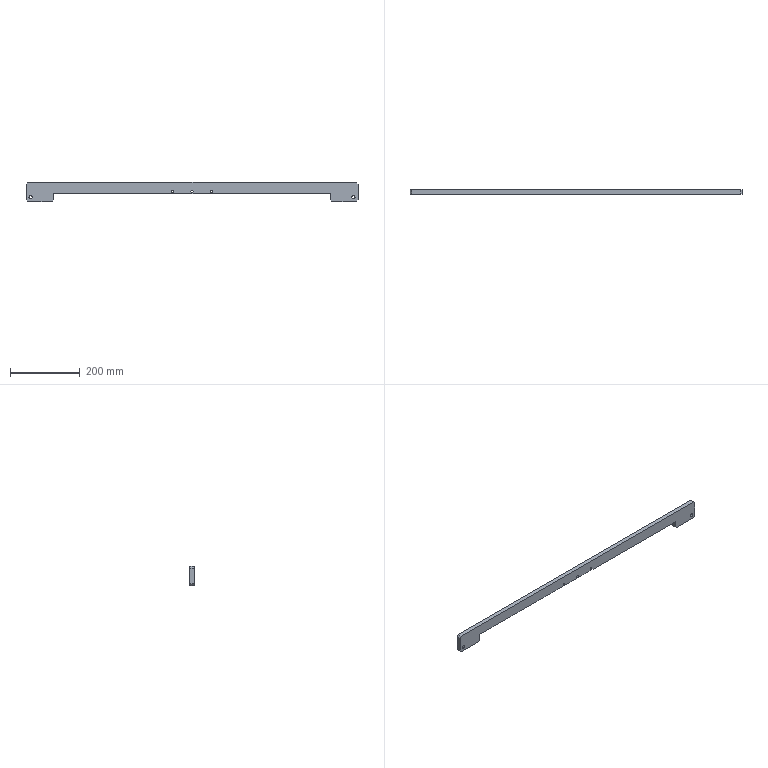Part | 1 solid | 35 faces | box 950 x 12 x 55 mm | volume 404061 mm3 | plane 19 | cylinder 16 | commonest cylinder face diameters 6.6 x6 11 x6 9 x4
STEP:
#1=CARTESIAN_POINT('',(55.,-0.8,-4.));
#2=VERTEX_POINT('',#1);
#3=CARTESIAN_POINT('',(55.,-0.8,7.));
#4=VERTEX_POINT('',#3);
#5=CARTESIAN_POINT('',(55.,-0.8,1.5));
#6=DIRECTION('',(0.,1.,0.));
#7=DIRECTION('',(0.,0.,1.));
#8=AXIS2_PLACEMENT_3D('',#5,#6,#7);
#9=CIRCLE('',#8,5.5);
#10=EDGE_CURVE('',#2,#4,#9,.T.);
#11=ORIENTED_EDGE('',*,*,#10,.F.);
#12=CARTESIAN_POINT('',(55.,6.,-4.));
#13=VERTEX_POINT('',#12);
#14=CARTESIAN_POINT('',(55.,6.,-4.));
#15=DIRECTION('',(0.,1.,0.));
#16=VECTOR('',#15,1000.);
#17=LINE('',#14,#16);
#18=EDGE_CURVE('',#2,#13,#17,.T.);
#19=ORIENTED_EDGE('',*,*,#18,.T.);
#20=CARTESIAN_POINT('',(55.,6.,7.));
#21=VERTEX_POINT('',#20);
#22=CARTESIAN_POINT('',(55.,6.,1.5));
#23=DIRECTION('',(0.,1.,0.));
#24=DIRECTION('',(0.,0.,1.));
#25=AXIS2_PLACEMENT_3D('',#22,#23,#24);
#26=CIRCLE('',#25,5.5);
#27=EDGE_CURVE('',#13,#21,#26,.T.);
#28=ORIENTED_EDGE('',*,*,#27,.T.);
#29=CARTESIAN_POINT('',(55.,6.,7.));
#30=DIRECTION('',(0.,1.,0.));
#31=VECTOR('',#30,1000.);
#32=LINE('',#29,#31);
#33=EDGE_CURVE('',#4,#21,#32,.T.);
#34=ORIENTED_EDGE('',*,*,#33,.F.);
#35=EDGE_LOOP('',(#11,#19,#28,#34));
#36=FACE_OUTER_BOUND('',#35,.T.);
#37=CARTESIAN_POINT('',(55.,6.,1.5));
#38=DIRECTION('',(0.,1.,0.));
#39=DIRECTION('',(0.,0.,1.));
#40=AXIS2_PLACEMENT_3D('',#37,#38,#39);
#41=CYLINDRICAL_SURFACE('',#40,5.5);
#42=ADVANCED_FACE('',(#36),#41,.F.);
#43=CARTESIAN_POINT('',(55.,-6.,-1.8));
#44=VERTEX_POINT('',#43);
#45=CARTESIAN_POINT('',(55.,-6.,4.8));
#46=VERTEX_POINT('',#45);
#47=CARTESIAN_POINT('',(55.,-6.,1.5));
#48=DIRECTION('',(0.,1.,0.));
#49=DIRECTION('',(0.,0.,1.));
#50=AXIS2_PLACEMENT_3D('',#47,#48,#49);
#51=CIRCLE('',#50,3.3);
#52=EDGE_CURVE('',#44,#46,#51,.T.);
#53=ORIENTED_EDGE('',*,*,#52,.F.);
#54=CARTESIAN_POINT('',(55.,-0.8,-1.8));
#55=VERTEX_POINT('',#54);
#56=CARTESIAN_POINT('',(55.,6.,-1.8));
#57=DIRECTION('',(0.,1.,0.));
#58=VECTOR('',#57,1000.);
#59=LINE('',#56,#58);
#60=EDGE_CURVE('',#44,#55,#59,.T.);
#61=ORIENTED_EDGE('',*,*,#60,.T.);
#62=CARTESIAN_POINT('',(55.,-0.8,4.8));
#63=VERTEX_POINT('',#62);
#64=CARTESIAN_POINT('',(55.,-0.8,1.5));
#65=DIRECTION('',(0.,1.,0.));
#66=DIRECTION('',(0.,0.,1.));
#67=AXIS2_PLACEMENT_3D('',#64,#65,#66);
#68=CIRCLE('',#67,3.3);
#69=EDGE_CURVE('',#55,#63,#68,.T.);
#70=ORIENTED_EDGE('',*,*,#69,.T.);
#71=CARTESIAN_POINT('',(55.,6.,4.8));
#72=DIRECTION('',(0.,1.,0.));
#73=VECTOR('',#72,1000.);
#74=LINE('',#71,#73);
#75=EDGE_CURVE('',#46,#63,#74,.T.);
#76=ORIENTED_EDGE('',*,*,#75,.F.);
#77=EDGE_LOOP('',(#53,#61,#70,#76));
#78=FACE_OUTER_BOUND('',#77,.T.);
#79=CARTESIAN_POINT('',(55.,6.,1.5));
#80=DIRECTION('',(0.,1.,0.));
#81=DIRECTION('',(0.,0.,1.));
#82=AXIS2_PLACEMENT_3D('',#79,#80,#81);
#83=CYLINDRICAL_SURFACE('',#82,3.3);
#84=ADVANCED_FACE('',(#78),#83,.F.);
#85=CARTESIAN_POINT('',(0.,-0.8,-4.));
#86=VERTEX_POINT('',#85);
#87=CARTESIAN_POINT('',(0.,-0.8,7.));
#88=VERTEX_POINT('',#87);
#89=CARTESIAN_POINT('',(0.,-0.8,1.5));
#90=DIRECTION('',(0.,1.,0.));
#91=DIRECTION('',(0.,0.,1.));
#92=AXIS2_PLACEMENT_3D('',#89,#90,#91);
#93=CIRCLE('',#92,5.5);
#94=EDGE_CURVE('',#86,#88,#93,.T.);
#95=ORIENTED_EDGE('',*,*,#94,.F.);
#96=CARTESIAN_POINT('',(0.,6.,-4.));
#97=VERTEX_POINT('',#96);
#98=CARTESIAN_POINT('',(0.,6.,-4.));
#99=DIRECTION('',(0.,1.,0.));
#100=VECTOR('',#99,1000.);
#101=LINE('',#98,#100);
#102=EDGE_CURVE('',#86,#97,#101,.T.);
#103=ORIENTED_EDGE('',*,*,#102,.T.);
#104=CARTESIAN_POINT('',(0.,6.,7.));
#105=VERTEX_POINT('',#104);
#106=CARTESIAN_POINT('',(0.,6.,1.5));
#107=DIRECTION('',(0.,1.,0.));
#108=DIRECTION('',(0.,0.,1.));
#109=AXIS2_PLACEMENT_3D('',#106,#107,#108);
#110=CIRCLE('',#109,5.5);
#111=EDGE_CURVE('',#97,#105,#110,.T.);
#112=ORIENTED_EDGE('',*,*,#111,.T.);
#113=CARTESIAN_POINT('',(0.,6.,7.));
#114=DIRECTION('',(0.,1.,0.));
#115=VECTOR('',#114,1000.);
#116=LINE('',#113,#115);
#117=EDGE_CURVE('',#88,#105,#116,.T.);
#118=ORIENTED_EDGE('',*,*,#117,.F.);
#119=EDGE_LOOP('',(#95,#103,#112,#118));
#120=FACE_OUTER_BOUND('',#119,.T.);
#121=CARTESIAN_POINT('',(0.,6.,1.5));
#122=DIRECTION('',(0.,1.,0.));
#123=DIRECTION('',(0.,0.,1.));
#124=AXIS2_PLACEMENT_3D('',#121,#122,#123);
#125=CYLINDRICAL_SURFACE('',#124,5.5);
#126=ADVANCED_FACE('',(#120),#125,.F.);
#127=CARTESIAN_POINT('',(0.,-6.,-1.8));
#128=VERTEX_POINT('',#127);
#129=CARTESIAN_POINT('',(0.,-6.,4.8));
#130=VERTEX_POINT('',#129);
#131=CARTESIAN_POINT('',(0.,-6.,1.5));
#132=DIRECTION('',(0.,1.,0.));
#133=DIRECTION('',(0.,0.,1.));
#134=AXIS2_PLACEMENT_3D('',#131,#132,#133);
#135=CIRCLE('',#134,3.3);
#136=EDGE_CURVE('',#128,#130,#135,.T.);
#137=ORIENTED_EDGE('',*,*,#136,.F.);
#138=CARTESIAN_POINT('',(0.,-0.8,-1.8));
#139=VERTEX_POINT('',#138);
#140=CARTESIAN_POINT('',(0.,6.,-1.8));
#141=DIRECTION('',(0.,1.,0.));
#142=VECTOR('',#141,1000.);
#143=LINE('',#140,#142);
#144=EDGE_CURVE('',#128,#139,#143,.T.);
#145=ORIENTED_EDGE('',*,*,#144,.T.);
#146=CARTESIAN_POINT('',(0.,-0.8,4.8));
#147=VERTEX_POINT('',#146);
#148=CARTESIAN_POINT('',(0.,-0.8,1.5));
#149=DIRECTION('',(0.,1.,0.));
#150=DIRECTION('',(0.,0.,1.));
#151=AXIS2_PLACEMENT_3D('',#148,#149,#150);
#152=CIRCLE('',#151,3.3);
#153=EDGE_CURVE('',#139,#147,#152,.T.);
#154=ORIENTED_EDGE('',*,*,#153,.T.);
#155=CARTESIAN_POINT('',(0.,6.,4.8));
#156=DIRECTION('',(0.,1.,0.));
#157=VECTOR('',#156,1000.);
#158=LINE('',#155,#157);
#159=EDGE_CURVE('',#130,#147,#158,.T.);
#160=ORIENTED_EDGE('',*,*,#159,.F.);
#161=EDGE_LOOP('',(#137,#145,#154,#160));
#162=FACE_OUTER_BOUND('',#161,.T.);
#163=CARTESIAN_POINT('',(0.,6.,1.5));
#164=DIRECTION('',(0.,1.,0.));
#165=DIRECTION('',(0.,0.,1.));
#166=AXIS2_PLACEMENT_3D('',#163,#164,#165);
#167=CYLINDRICAL_SURFACE('',#166,3.3);
#168=ADVANCED_FACE('',(#162),#167,.F.);
#169=CARTESIAN_POINT('',(-55.,-0.8,-4.));
#170=VERTEX_POINT('',#169);
#171=CARTESIAN_POINT('',(-55.,-0.8,7.));
#172=VERTEX_POINT('',#171);
#173=CARTESIAN_POINT('',(-55.,-0.8,1.5));
#174=DIRECTION('',(0.,1.,0.));
#175=DIRECTION('',(0.,0.,1.));
#176=AXIS2_PLACEMENT_3D('',#173,#174,#175);
#177=CIRCLE('',#176,5.5);
#178=EDGE_CURVE('',#170,#172,#177,.T.);
#179=ORIENTED_EDGE('',*,*,#178,.F.);
#180=CARTESIAN_POINT('',(-55.,6.,-4.));
#181=VERTEX_POINT('',#180);
#182=CARTESIAN_POINT('',(-55.,6.,-4.));
#183=DIRECTION('',(0.,1.,0.));
#184=VECTOR('',#183,1000.);
#185=LINE('',#182,#184);
#186=EDGE_CURVE('',#170,#181,#185,.T.);
#187=ORIENTED_EDGE('',*,*,#186,.T.);
#188=CARTESIAN_POINT('',(-55.,6.,7.));
#189=VERTEX_POINT('',#188);
#190=CARTESIAN_POINT('',(-55.,6.,1.5));
#191=DIRECTION('',(0.,1.,0.));
#192=DIRECTION('',(0.,0.,1.));
#193=AXIS2_PLACEMENT_3D('',#190,#191,#192);
#194=CIRCLE('',#193,5.5);
#195=EDGE_CURVE('',#181,#189,#194,.T.);
#196=ORIENTED_EDGE('',*,*,#195,.T.);
#197=CARTESIAN_POINT('',(-55.,6.,7.));
#198=DIRECTION('',(0.,1.,0.));
#199=VECTOR('',#198,1000.);
#200=LINE('',#197,#199);
#201=EDGE_CURVE('',#172,#189,#200,.T.);
#202=ORIENTED_EDGE('',*,*,#201,.F.);
#203=EDGE_LOOP('',(#179,#187,#196,#202));
#204=FACE_OUTER_BOUND('',#203,.T.);
#205=CARTESIAN_POINT('',(-55.,6.,1.5));
#206=DIRECTION('',(0.,1.,0.));
#207=DIRECTION('',(0.,0.,1.));
#208=AXIS2_PLACEMENT_3D('',#205,#206,#207);
#209=CYLINDRICAL_SURFACE('',#208,5.5);
#210=ADVANCED_FACE('',(#204),#209,.F.);
#211=CARTESIAN_POINT('',(-55.,-6.,-1.8));
#212=VERTEX_POINT('',#211);
#213=CARTESIAN_POINT('',(-55.,-6.,4.8));
#214=VERTEX_POINT('',#213);
#215=CARTESIAN_POINT('',(-55.,-6.,1.5));
#216=DIRECTION('',(0.,1.,0.));
#217=DIRECTION('',(0.,0.,1.));
#218=AXIS2_PLACEMENT_3D('',#215,#216,#217);
#219=CIRCLE('',#218,3.3);
#220=EDGE_CURVE('',#212,#214,#219,.T.);
#221=ORIENTED_EDGE('',*,*,#220,.F.);
#222=CARTESIAN_POINT('',(-55.,-0.8,-1.8));
#223=VERTEX_POINT('',#222);
#224=CARTESIAN_POINT('',(-55.,6.,-1.8));
#225=DIRECTION('',(0.,1.,0.));
#226=VECTOR('',#225,1000.);
#227=LINE('',#224,#226);
#228=EDGE_CURVE('',#212,#223,#227,.T.);
#229=ORIENTED_EDGE('',*,*,#228,.T.);
#230=CARTESIAN_POINT('',(-55.,-0.8,4.8));
#231=VERTEX_POINT('',#230);
#232=CARTESIAN_POINT('',(-55.,-0.8,1.5));
#233=DIRECTION('',(0.,1.,0.));
#234=DIRECTION('',(0.,0.,1.));
#235=AXIS2_PLACEMENT_3D('',#232,#233,#234);
#236=CIRCLE('',#235,3.3);
#237=EDGE_CURVE('',#223,#231,#236,.T.);
#238=ORIENTED_EDGE('',*,*,#237,.T.);
#239=CARTESIAN_POINT('',(-55.,6.,4.8));
#240=DIRECTION('',(0.,1.,0.));
#241=VECTOR('',#240,1000.);
#242=LINE('',#239,#241);
#243=EDGE_CURVE('',#214,#231,#242,.T.);
#244=ORIENTED_EDGE('',*,*,#243,.F.);
#245=EDGE_LOOP('',(#221,#229,#238,#244));
#246=FACE_OUTER_BOUND('',#245,.T.);
#247=CARTESIAN_POINT('',(-55.,6.,1.5));
#248=DIRECTION('',(0.,1.,0.));
#249=DIRECTION('',(0.,0.,1.));
#250=AXIS2_PLACEMENT_3D('',#247,#248,#249);
#251=CYLINDRICAL_SURFACE('',#250,3.3);
#252=ADVANCED_FACE('',(#246),#251,.F.);
#253=CARTESIAN_POINT('',(-462.,6.,-10.5));
#254=VERTEX_POINT('',#253);
#255=CARTESIAN_POINT('',(-462.,6.,-19.5));
#256=VERTEX_POINT('',#255);
#257=CARTESIAN_POINT('',(-462.,6.,-15.));
#258=DIRECTION('',(0.,-1.,0.));
#259=DIRECTION('',(0.,0.,-1.));
#260=AXIS2_PLACEMENT_3D('',#257,#258,#259);
#261=CIRCLE('',#260,4.5);
#262=EDGE_CURVE('',#254,#256,#261,.T.);
#263=ORIENTED_EDGE('',*,*,#262,.F.);
#264=CARTESIAN_POINT('',(-462.,-6.,-10.5));
#265=VERTEX_POINT('',#264);
#266=CARTESIAN_POINT('',(-462.,-6.,-10.5));
#267=DIRECTION('',(0.,-1.,0.));
#268=VECTOR('',#267,1000.);
#269=LINE('',#266,#268);
#270=EDGE_CURVE('',#254,#265,#269,.T.);
#271=ORIENTED_EDGE('',*,*,#270,.T.);
#272=CARTESIAN_POINT('',(-462.,-6.,-19.5));
#273=VERTEX_POINT('',#272);
#274=CARTESIAN_POINT('',(-462.,-6.,-15.));
#275=DIRECTION('',(0.,-1.,0.));
#276=DIRECTION('',(0.,0.,-1.));
#277=AXIS2_PLACEMENT_3D('',#274,#275,#276);
#278=CIRCLE('',#277,4.5);
#279=EDGE_CURVE('',#265,#273,#278,.T.);
#280=ORIENTED_EDGE('',*,*,#279,.T.);
#281=CARTESIAN_POINT('',(-462.,-6.,-19.5));
#282=DIRECTION('',(0.,-1.,0.));
#283=VECTOR('',#282,1000.);
#284=LINE('',#281,#283);
#285=EDGE_CURVE('',#256,#273,#284,.T.);
#286=ORIENTED_EDGE('',*,*,#285,.F.);
#287=EDGE_LOOP('',(#263,#271,#280,#286));
#288=FACE_OUTER_BOUND('',#287,.T.);
#289=CARTESIAN_POINT('',(-462.,-6.,-15.));
#290=DIRECTION('',(0.,-1.,0.));
#291=DIRECTION('',(0.,0.,-1.));
#292=AXIS2_PLACEMENT_3D('',#289,#290,#291);
#293=CYLINDRICAL_SURFACE('',#292,4.5);
#294=ADVANCED_FACE('',(#288),#293,.F.);
#295=CARTESIAN_POINT('',(462.,6.,-10.5));
#296=VERTEX_POINT('',#295);
#297=CARTESIAN_POINT('',(462.,6.,-19.5));
#298=VERTEX_POINT('',#297);
#299=CARTESIAN_POINT('',(462.,6.,-15.));
#300=DIRECTION('',(0.,-1.,0.));
#301=DIRECTION('',(0.,0.,-1.));
#302=AXIS2_PLACEMENT_3D('',#299,#300,#301);
#303=CIRCLE('',#302,4.5);
#304=EDGE_CURVE('',#296,#298,#303,.T.);
#305=ORIENTED_EDGE('',*,*,#304,.F.);
#306=CARTESIAN_POINT('',(462.,-6.,-10.5));
#307=VERTEX_POINT('',#306);
#308=CARTESIAN_POINT('',(462.,-6.,-10.5));
#309=DIRECTION('',(0.,-1.,0.));
#310=VECTOR('',#309,1000.);
#311=LINE('',#308,#310);
#312=EDGE_CURVE('',#296,#307,#311,.T.);
#313=ORIENTED_EDGE('',*,*,#312,.T.);
#314=CARTESIAN_POINT('',(462.,-6.,-19.5));
#315=VERTEX_POINT('',#314);
#316=CARTESIAN_POINT('',(462.,-6.,-15.));
#317=DIRECTION('',(0.,-1.,0.));
#318=DIRECTION('',(0.,0.,-1.));
#319=AXIS2_PLACEMENT_3D('',#316,#317,#318);
#320=CIRCLE('',#319,4.5);
#321=EDGE_CURVE('',#307,#315,#320,.T.);
#322=ORIENTED_EDGE('',*,*,#321,.T.);
#323=CARTESIAN_POINT('',(462.,-6.,-19.5));
#324=DIRECTION('',(0.,-1.,0.));
#325=VECTOR('',#324,1000.);
#326=LINE('',#323,#325);
#327=EDGE_CURVE('',#298,#315,#326,.T.);
#328=ORIENTED_EDGE('',*,*,#327,.F.);
#329=EDGE_LOOP('',(#305,#313,#322,#328));
#330=FACE_OUTER_BOUND('',#329,.T.);
#331=CARTESIAN_POINT('',(462.,-6.,-15.));
#332=DIRECTION('',(0.,-1.,0.));
#333=DIRECTION('',(0.,0.,-1.));
#334=AXIS2_PLACEMENT_3D('',#331,#332,#333);
#335=CYLINDRICAL_SURFACE('',#334,4.5);
#336=ADVANCED_FACE('',(#330),#335,.F.);
#337=CARTESIAN_POINT('',(-475.,-6.,-22.5));
#338=VERTEX_POINT('',#337);
#339=CARTESIAN_POINT('',(-475.,-6.,22.5));
#340=VERTEX_POINT('',#339);
#341=CARTESIAN_POINT('',(-475.,-6.,27.5));
#342=DIRECTION('',(0.,0.,1.));
#343=VECTOR('',#342,1000.);
#344=LINE('',#341,#343);
#345=EDGE_CURVE('',#338,#340,#344,.T.);
#346=ORIENTED_EDGE('',*,*,#345,.F.);
#347=CARTESIAN_POINT('',(-470.,-6.,-27.5));
#348=VERTEX_POINT('',#347);
#349=CARTESIAN_POINT('',(-248.75,-6.,-248.75));
#350=DIRECTION('',(0.7071,0.,-0.7071));
#351=VECTOR('',#350,1000.);
#352=LINE('',#349,#351);
#353=EDGE_CURVE('',#338,#348,#352,.T.);
#354=ORIENTED_EDGE('',*,*,#353,.T.);
#355=CARTESIAN_POINT('',(-400.,-6.,-27.5));
#356=VERTEX_POINT('',#355);
#357=CARTESIAN_POINT('',(-475.,-6.,-27.5));
#358=DIRECTION('',(-1.,0.,0.));
#359=VECTOR('',#358,1000.);
#360=LINE('',#357,#359);
#361=EDGE_CURVE('',#356,#348,#360,.T.);
#362=ORIENTED_EDGE('',*,*,#361,.F.);
#363=CARTESIAN_POINT('',(-395.,-6.,-22.5));
#364=VERTEX_POINT('',#363);
#365=CARTESIAN_POINT('',(-186.25,-6.,186.25));
#366=DIRECTION('',(0.7071,0.,0.7071));
#367=VECTOR('',#366,1000.);
#368=LINE('',#365,#367);
#369=EDGE_CURVE('',#356,#364,#368,.T.);
#370=ORIENTED_EDGE('',*,*,#369,.T.);
#371=CARTESIAN_POINT('',(-395.,-6.,-4.5));
#372=VERTEX_POINT('',#371);
#373=CARTESIAN_POINT('',(-395.,-6.,-27.5));
#374=DIRECTION('',(0.,0.,1.));
#375=VECTOR('',#374,1000.);
#376=LINE('',#373,#375);
#377=EDGE_CURVE('',#364,#372,#376,.T.);
#378=ORIENTED_EDGE('',*,*,#377,.T.);
#379=CARTESIAN_POINT('',(395.,-6.,-4.5));
#380=VERTEX_POINT('',#379);
#381=CARTESIAN_POINT('',(395.,-6.,-4.5));
#382=DIRECTION('',(1.,0.,0.));
#383=VECTOR('',#382,1000.);
#384=LINE('',#381,#383);
#385=EDGE_CURVE('',#372,#380,#384,.T.);
#386=ORIENTED_EDGE('',*,*,#385,.T.);
#387=CARTESIAN_POINT('',(395.,-6.,-22.5));
#388=VERTEX_POINT('',#387);
#389=CARTESIAN_POINT('',(395.,-6.,-27.5));
#390=DIRECTION('',(0.,0.,-1.));
#391=VECTOR('',#390,1000.);
#392=LINE('',#389,#391);
#393=EDGE_CURVE('',#380,#388,#392,.T.);
#394=ORIENTED_EDGE('',*,*,#393,.T.);
#395=CARTESIAN_POINT('',(400.,-6.,-27.5));
#396=VERTEX_POINT('',#395);
#397=CARTESIAN_POINT('',(186.25,-6.,186.25));
#398=DIRECTION('',(0.7071,0.,-0.7071));
#399=VECTOR('',#398,1000.);
#400=LINE('',#397,#399);
#401=EDGE_CURVE('',#388,#396,#400,.T.);
#402=ORIENTED_EDGE('',*,*,#401,.T.);
#403=CARTESIAN_POINT('',(470.,-6.,-27.5));
#404=VERTEX_POINT('',#403);
#405=CARTESIAN_POINT('',(-475.,-6.,-27.5));
#406=DIRECTION('',(-1.,0.,0.));
#407=VECTOR('',#406,1000.);
#408=LINE('',#405,#407);
#409=EDGE_CURVE('',#404,#396,#408,.T.);
#410=ORIENTED_EDGE('',*,*,#409,.F.);
#411=CARTESIAN_POINT('',(475.,-6.,-22.5));
#412=VERTEX_POINT('',#411);
#413=CARTESIAN_POINT('',(248.75,-6.,-248.75));
#414=DIRECTION('',(0.7071,0.,0.7071));
#415=VECTOR('',#414,1000.);
#416=LINE('',#413,#415);
#417=EDGE_CURVE('',#404,#412,#416,.T.);
#418=ORIENTED_EDGE('',*,*,#417,.T.);
#419=CARTESIAN_POINT('',(475.,-6.,22.5));
#420=VERTEX_POINT('',#419);
#421=CARTESIAN_POINT('',(475.,-6.,27.5));
#422=DIRECTION('',(0.,0.,-1.));
#423=VECTOR('',#422,1000.);
#424=LINE('',#421,#423);
#425=EDGE_CURVE('',#420,#412,#424,.T.);
#426=ORIENTED_EDGE('',*,*,#425,.F.);
#427=CARTESIAN_POINT('',(470.,-6.,27.5));
#428=VERTEX_POINT('',#427);
#429=CARTESIAN_POINT('',(248.75,-6.,248.75));
#430=DIRECTION('',(-0.7071,0.,0.7071));
#431=VECTOR('',#430,1000.);
#432=LINE('',#429,#431);
#433=EDGE_CURVE('',#420,#428,#432,.T.);
#434=ORIENTED_EDGE('',*,*,#433,.T.);
#435=CARTESIAN_POINT('',(-470.,-6.,27.5));
#436=VERTEX_POINT('',#435);
#437=CARTESIAN_POINT('',(-475.,-6.,27.5));
#438=DIRECTION('',(1.,0.,0.));
#439=VECTOR('',#438,1000.);
#440=LINE('',#437,#439);
#441=EDGE_CURVE('',#436,#428,#440,.T.);
#442=ORIENTED_EDGE('',*,*,#441,.F.);
#443=CARTESIAN_POINT('',(-248.75,-6.,248.75));
#444=DIRECTION('',(-0.7071,0.,-0.7071));
#445=VECTOR('',#444,1000.);
#446=LINE('',#443,#445);
#447=EDGE_CURVE('',#436,#340,#446,.T.);
#448=ORIENTED_EDGE('',*,*,#447,.T.);
#449=EDGE_LOOP('',(#346,#354,#362,#370,#378,#386,#394,#402,#410,#418,#426,#434,#442,#448));
#450=FACE_OUTER_BOUND('',#449,.T.);
#451=CARTESIAN_POINT('',(462.,-6.,-15.));
#452=DIRECTION('',(0.,-1.,0.));
#453=DIRECTION('',(0.,0.,-1.));
#454=AXIS2_PLACEMENT_3D('',#451,#452,#453);
#455=CIRCLE('',#454,4.5);
#456=EDGE_CURVE('',#315,#307,#455,.T.);
#457=ORIENTED_EDGE('',*,*,#456,.F.);
#458=ORIENTED_EDGE('',*,*,#321,.F.);
#459=EDGE_LOOP('',(#457,#458));
#460=FACE_BOUND('',#459,.T.);
#461=CARTESIAN_POINT('',(-462.,-6.,-15.));
#462=DIRECTION('',(0.,-1.,0.));
#463=DIRECTION('',(0.,0.,-1.));
#464=AXIS2_PLACEMENT_3D('',#461,#462,#463);
#465=CIRCLE('',#464,4.5);
#466=EDGE_CURVE('',#273,#265,#465,.T.);
#467=ORIENTED_EDGE('',*,*,#466,.F.);
#468=ORIENTED_EDGE('',*,*,#279,.F.);
#469=EDGE_LOOP('',(#467,#468));
#470=FACE_BOUND('',#469,.T.);
#471=CARTESIAN_POINT('',(-55.,-6.,1.5));
#472=DIRECTION('',(0.,1.,0.));
#473=DIRECTION('',(0.,0.,1.));
#474=AXIS2_PLACEMENT_3D('',#471,#472,#473);
#475=CIRCLE('',#474,3.3);
#476=EDGE_CURVE('',#214,#212,#475,.T.);
#477=ORIENTED_EDGE('',*,*,#476,.T.);
#478=ORIENTED_EDGE('',*,*,#220,.T.);
#479=EDGE_LOOP('',(#477,#478));
#480=FACE_BOUND('',#479,.T.);
#481=CARTESIAN_POINT('',(0.,-6.,1.5));
#482=DIRECTION('',(0.,1.,0.));
#483=DIRECTION('',(0.,0.,1.));
#484=AXIS2_PLACEMENT_3D('',#481,#482,#483);
#485=CIRCLE('',#484,3.3);
#486=EDGE_CURVE('',#130,#128,#485,.T.);
#487=ORIENTED_EDGE('',*,*,#486,.T.);
#488=ORIENTED_EDGE('',*,*,#136,.T.);
#489=EDGE_LOOP('',(#487,#488));
#490=FACE_BOUND('',#489,.T.);
#491=CARTESIAN_POINT('',(55.,-6.,1.5));
#492=DIRECTION('',(0.,1.,0.));
#493=DIRECTION('',(0.,0.,1.));
#494=AXIS2_PLACEMENT_3D('',#491,#492,#493);
#495=CIRCLE('',#494,3.3);
#496=EDGE_CURVE('',#46,#44,#495,.T.);
#497=ORIENTED_EDGE('',*,*,#496,.T.);
#498=ORIENTED_EDGE('',*,*,#52,.T.);
#499=EDGE_LOOP('',(#497,#498));
#500=FACE_BOUND('',#499,.T.);
#501=CARTESIAN_POINT('',(0.,-6.,0.));
#502=DIRECTION('',(0.,-1.,0.));
#503=DIRECTION('',(0.,0.,-1.));
#504=AXIS2_PLACEMENT_3D('',#501,#502,#503);
#505=PLANE('',#504);
#506=ADVANCED_FACE('',(#450,#460,#470,#480,#490,#500),#505,.T.);
#507=ORIENTED_EDGE('',*,*,#361,.T.);
#508=CARTESIAN_POINT('',(-470.,6.,-27.5));
#509=VERTEX_POINT('',#508);
#510=CARTESIAN_POINT('',(-470.,6.,-27.5));
#511=DIRECTION('',(0.,1.,0.));
#512=VECTOR('',#511,1000.);
#513=LINE('',#510,#512);
#514=EDGE_CURVE('',#348,#509,#513,.T.);
#515=ORIENTED_EDGE('',*,*,#514,.T.);
#516=CARTESIAN_POINT('',(-400.,6.,-27.5));
#517=VERTEX_POINT('',#516);
#518=CARTESIAN_POINT('',(-475.,6.,-27.5));
#519=DIRECTION('',(-1.,0.,0.));
#520=VECTOR('',#519,1000.);
#521=LINE('',#518,#520);
#522=EDGE_CURVE('',#517,#509,#521,.T.);
#523=ORIENTED_EDGE('',*,*,#522,.F.);
#524=CARTESIAN_POINT('',(-400.,6.,-27.5));
#525=DIRECTION('',(0.,-1.,0.));
#526=VECTOR('',#525,1000.);
#527=LINE('',#524,#526);
#528=EDGE_CURVE('',#517,#356,#527,.T.);
#529=ORIENTED_EDGE('',*,*,#528,.T.);
#530=EDGE_LOOP('',(#507,#515,#523,#529));
#531=FACE_OUTER_BOUND('',#530,.T.);
#532=CARTESIAN_POINT('',(-475.,6.,-27.5));
#533=DIRECTION('',(0.,0.,1.));
#534=DIRECTION('',(1.,0.,0.));
#535=AXIS2_PLACEMENT_3D('',#532,#533,#534);
#536=PLANE('',#535);
#537=ADVANCED_FACE('',(#531),#536,.F.);
#538=ORIENTED_EDGE('',*,*,#425,.T.);
#539=CARTESIAN_POINT('',(475.,6.,-22.5));
#540=VERTEX_POINT('',#539);
#541=CARTESIAN_POINT('',(475.,6.,-22.5));
#542=DIRECTION('',(0.,1.,0.));
#543=VECTOR('',#542,1000.);
#544=LINE('',#541,#543);
#545=EDGE_CURVE('',#412,#540,#544,.T.);
#546=ORIENTED_EDGE('',*,*,#545,.T.);
#547=CARTESIAN_POINT('',(475.,6.,22.5));
#548=VERTEX_POINT('',#547);
#549=CARTESIAN_POINT('',(475.,6.,27.5));
#550=DIRECTION('',(0.,0.,-1.));
#551=VECTOR('',#550,1000.);
#552=LINE('',#549,#551);
#553=EDGE_CURVE('',#548,#540,#552,.T.);
#554=ORIENTED_EDGE('',*,*,#553,.F.);
#555=CARTESIAN_POINT('',(475.,6.,22.5));
#556=DIRECTION('',(0.,-1.,0.));
#557=VECTOR('',#556,1000.);
#558=LINE('',#555,#557);
#559=EDGE_CURVE('',#548,#420,#558,.T.);
#560=ORIENTED_EDGE('',*,*,#559,.T.);
#561=EDGE_LOOP('',(#538,#546,#554,#560));
#562=FACE_OUTER_BOUND('',#561,.T.);
#563=CARTESIAN_POINT('',(475.,6.,27.5));
#564=DIRECTION('',(-1.,0.,0.));
#565=DIRECTION('',(0.,0.,1.));
#566=AXIS2_PLACEMENT_3D('',#563,#564,#565);
#567=PLANE('',#566);
#568=ADVANCED_FACE('',(#562),#567,.F.);
#569=ORIENTED_EDGE('',*,*,#409,.T.);
#570=CARTESIAN_POINT('',(400.,6.,-27.5));
#571=VERTEX_POINT('',#570);
#572=CARTESIAN_POINT('',(400.,6.,-27.5));
#573=DIRECTION('',(0.,1.,0.));
#574=VECTOR('',#573,1000.);
#575=LINE('',#572,#574);
#576=EDGE_CURVE('',#396,#571,#575,.T.);
#577=ORIENTED_EDGE('',*,*,#576,.T.);
#578=CARTESIAN_POINT('',(470.,6.,-27.5));
#579=VERTEX_POINT('',#578);
#580=CARTESIAN_POINT('',(-475.,6.,-27.5));
#581=DIRECTION('',(-1.,0.,0.));
#582=VECTOR('',#581,1000.);
#583=LINE('',#580,#582);
#584=EDGE_CURVE('',#579,#571,#583,.T.);
#585=ORIENTED_EDGE('',*,*,#584,.F.);
#586=CARTESIAN_POINT('',(470.,6.,-27.5));
#587=DIRECTION('',(0.,-1.,0.));
#588=VECTOR('',#587,1000.);
#589=LINE('',#586,#588);
#590=EDGE_CURVE('',#579,#404,#589,.T.);
#591=ORIENTED_EDGE('',*,*,#590,.T.);
#592=EDGE_LOOP('',(#569,#577,#585,#591));
#593=FACE_OUTER_BOUND('',#592,.T.);
#594=CARTESIAN_POINT('',(-475.,6.,-27.5));
#595=DIRECTION('',(0.,0.,1.));
#596=DIRECTION('',(1.,0.,0.));
#597=AXIS2_PLACEMENT_3D('',#594,#595,#596);
#598=PLANE('',#597);
#599=ADVANCED_FACE('',(#593),#598,.F.);
#600=CARTESIAN_POINT('',(-475.,6.,-22.5));
#601=VERTEX_POINT('',#600);
#602=CARTESIAN_POINT('',(-475.,6.,22.5));
#603=VERTEX_POINT('',#602);
#604=CARTESIAN_POINT('',(-475.,6.,27.5));
#605=DIRECTION('',(0.,0.,1.));
#606=VECTOR('',#605,1000.);
#607=LINE('',#604,#606);
#608=EDGE_CURVE('',#601,#603,#607,.T.);
#609=ORIENTED_EDGE('',*,*,#608,.F.);
#610=CARTESIAN_POINT('',(-475.,6.,-22.5));
#611=DIRECTION('',(0.,-1.,0.));
#612=VECTOR('',#611,1000.);
#613=LINE('',#610,#612);
#614=EDGE_CURVE('',#601,#338,#613,.T.);
#615=ORIENTED_EDGE('',*,*,#614,.T.);
#616=ORIENTED_EDGE('',*,*,#345,.T.);
#617=CARTESIAN_POINT('',(-475.,6.,22.5));
#618=DIRECTION('',(0.,1.,0.));
#619=VECTOR('',#618,1000.);
#620=LINE('',#617,#619);
#621=EDGE_CURVE('',#340,#603,#620,.T.);
#622=ORIENTED_EDGE('',*,*,#621,.T.);
#623=EDGE_LOOP('',(#609,#615,#616,#622));
#624=FACE_OUTER_BOUND('',#623,.T.);
#625=CARTESIAN_POINT('',(-475.,6.,27.5));
#626=DIRECTION('',(1.,0.,0.));
#627=DIRECTION('',(0.,0.,-1.));
#628=AXIS2_PLACEMENT_3D('',#625,#626,#627);
#629=PLANE('',#628);
#630=ADVANCED_FACE('',(#624),#629,.F.);
#631=CARTESIAN_POINT('',(-470.,6.,27.5));
#632=VERTEX_POINT('',#631);
#633=CARTESIAN_POINT('',(470.,6.,27.5));
#634=VERTEX_POINT('',#633);
#635=CARTESIAN_POINT('',(-475.,6.,27.5));
#636=DIRECTION('',(1.,0.,0.));
#637=VECTOR('',#636,1000.);
#638=LINE('',#635,#637);
#639=EDGE_CURVE('',#632,#634,#638,.T.);
#640=ORIENTED_EDGE('',*,*,#639,.F.);
#641=CARTESIAN_POINT('',(-470.,6.,27.5));
#642=DIRECTION('',(0.,-1.,0.));
#643=VECTOR('',#642,1000.);
#644=LINE('',#641,#643);
#645=EDGE_CURVE('',#632,#436,#644,.T.);
#646=ORIENTED_EDGE('',*,*,#645,.T.);
#647=ORIENTED_EDGE('',*,*,#441,.T.);
#648=CARTESIAN_POINT('',(470.,6.,27.5));
#649=DIRECTION('',(0.,1.,0.));
#650=VECTOR('',#649,1000.);
#651=LINE('',#648,#650);
#652=EDGE_CURVE('',#428,#634,#651,.T.);
#653=ORIENTED_EDGE('',*,*,#652,.T.);
#654=EDGE_LOOP('',(#640,#646,#647,#653));
#655=FACE_OUTER_BOUND('',#654,.T.);
#656=CARTESIAN_POINT('',(-475.,6.,27.5));
#657=DIRECTION('',(0.,0.,-1.));
#658=DIRECTION('',(-1.,0.,0.));
#659=AXIS2_PLACEMENT_3D('',#656,#657,#658);
#660=PLANE('',#659);
#661=ADVANCED_FACE('',(#655),#660,.F.);
#662=CARTESIAN_POINT('',(55.,6.,1.5));
#663=DIRECTION('',(0.,1.,0.));
#664=DIRECTION('',(0.,0.,1.));
#665=AXIS2_PLACEMENT_3D('',#662,#663,#664);
#666=CIRCLE('',#665,5.5);
#667=EDGE_CURVE('',#21,#13,#666,.T.);
#668=ORIENTED_EDGE('',*,*,#667,.F.);
#669=ORIENTED_EDGE('',*,*,#27,.F.);
#670=EDGE_LOOP('',(#668,#669));
#671=FACE_BOUND('',#670,.T.);
#672=CARTESIAN_POINT('',(0.,6.,1.5));
#673=DIRECTION('',(0.,1.,0.));
#674=DIRECTION('',(0.,0.,1.));
#675=AXIS2_PLACEMENT_3D('',#672,#673,#674);
#676=CIRCLE('',#675,5.5);
#677=EDGE_CURVE('',#105,#97,#676,.T.);
#678=ORIENTED_EDGE('',*,*,#677,.F.);
#679=ORIENTED_EDGE('',*,*,#111,.F.);
#680=EDGE_LOOP('',(#678,#679));
#681=FACE_BOUND('',#680,.T.);
#682=CARTESIAN_POINT('',(-55.,6.,1.5));
#683=DIRECTION('',(0.,1.,0.));
#684=DIRECTION('',(0.,0.,1.));
#685=AXIS2_PLACEMENT_3D('',#682,#683,#684);
#686=CIRCLE('',#685,5.5);
#687=EDGE_CURVE('',#189,#181,#686,.T.);
#688=ORIENTED_EDGE('',*,*,#687,.F.);
#689=ORIENTED_EDGE('',*,*,#195,.F.);
#690=EDGE_LOOP('',(#688,#689));
#691=FACE_BOUND('',#690,.T.);
#692=CARTESIAN_POINT('',(-462.,6.,-15.));
#693=DIRECTION('',(0.,-1.,0.));
#694=DIRECTION('',(0.,0.,-1.));
#695=AXIS2_PLACEMENT_3D('',#692,#693,#694);
#696=CIRCLE('',#695,4.5);
#697=EDGE_CURVE('',#256,#254,#696,.T.);
#698=ORIENTED_EDGE('',*,*,#697,.T.);
#699=ORIENTED_EDGE('',*,*,#262,.T.);
#700=EDGE_LOOP('',(#698,#699));
#701=FACE_BOUND('',#700,.T.);
#702=CARTESIAN_POINT('',(462.,6.,-15.));
#703=DIRECTION('',(0.,-1.,0.));
#704=DIRECTION('',(0.,0.,-1.));
#705=AXIS2_PLACEMENT_3D('',#702,#703,#704);
#706=CIRCLE('',#705,4.5);
#707=EDGE_CURVE('',#298,#296,#706,.T.);
#708=ORIENTED_EDGE('',*,*,#707,.T.);
#709=ORIENTED_EDGE('',*,*,#304,.T.);
#710=EDGE_LOOP('',(#708,#709));
#711=FACE_BOUND('',#710,.T.);
#712=ORIENTED_EDGE('',*,*,#522,.T.);
#713=CARTESIAN_POINT('',(-475.,6.,-22.5));
#714=DIRECTION('',(-0.7071,0.,0.7071));
#715=VECTOR('',#714,1000.);
#716=LINE('',#713,#715);
#717=EDGE_CURVE('',#509,#601,#716,.T.);
#718=ORIENTED_EDGE('',*,*,#717,.T.);
#719=ORIENTED_EDGE('',*,*,#608,.T.);
#720=CARTESIAN_POINT('',(-470.,6.,27.5));
#721=DIRECTION('',(0.7071,0.,0.7071));
#722=VECTOR('',#721,1000.);
#723=LINE('',#720,#722);
#724=EDGE_CURVE('',#603,#632,#723,.T.);
#725=ORIENTED_EDGE('',*,*,#724,.T.);
#726=ORIENTED_EDGE('',*,*,#639,.T.);
#727=CARTESIAN_POINT('',(475.,6.,22.5));
#728=DIRECTION('',(0.7071,0.,-0.7071));
#729=VECTOR('',#728,1000.);
#730=LINE('',#727,#729);
#731=EDGE_CURVE('',#634,#548,#730,.T.);
#732=ORIENTED_EDGE('',*,*,#731,.T.);
#733=ORIENTED_EDGE('',*,*,#553,.T.);
#734=CARTESIAN_POINT('',(470.,6.,-27.5));
#735=DIRECTION('',(-0.7071,0.,-0.7071));
#736=VECTOR('',#735,1000.);
#737=LINE('',#734,#736);
#738=EDGE_CURVE('',#540,#579,#737,.T.);
#739=ORIENTED_EDGE('',*,*,#738,.T.);
#740=ORIENTED_EDGE('',*,*,#584,.T.);
#741=CARTESIAN_POINT('',(395.,6.,-22.5));
#742=VERTEX_POINT('',#741);
#743=CARTESIAN_POINT('',(400.,6.,-27.5));
#744=DIRECTION('',(-0.7071,0.,0.7071));
#745=VECTOR('',#744,1000.);
#746=LINE('',#743,#745);
#747=EDGE_CURVE('',#571,#742,#746,.T.);
#748=ORIENTED_EDGE('',*,*,#747,.T.);
#749=CARTESIAN_POINT('',(395.,6.,-4.5));
#750=VERTEX_POINT('',#749);
#751=CARTESIAN_POINT('',(395.,6.,-27.5));
#752=DIRECTION('',(0.,0.,-1.));
#753=VECTOR('',#752,1000.);
#754=LINE('',#751,#753);
#755=EDGE_CURVE('',#750,#742,#754,.T.);
#756=ORIENTED_EDGE('',*,*,#755,.F.);
#757=CARTESIAN_POINT('',(-395.,6.,-4.5));
#758=VERTEX_POINT('',#757);
#759=CARTESIAN_POINT('',(395.,6.,-4.5));
#760=DIRECTION('',(1.,0.,0.));
#761=VECTOR('',#760,1000.);
#762=LINE('',#759,#761);
#763=EDGE_CURVE('',#758,#750,#762,.T.);
#764=ORIENTED_EDGE('',*,*,#763,.F.);
#765=CARTESIAN_POINT('',(-395.,6.,-22.5));
#766=VERTEX_POINT('',#765);
#767=CARTESIAN_POINT('',(-395.,6.,-27.5));
#768=DIRECTION('',(0.,0.,1.));
#769=VECTOR('',#768,1000.);
#770=LINE('',#767,#769);
#771=EDGE_CURVE('',#766,#758,#770,.T.);
#772=ORIENTED_EDGE('',*,*,#771,.F.);
#773=CARTESIAN_POINT('',(-395.,6.,-22.5));
#774=DIRECTION('',(-0.7071,0.,-0.7071));
#775=VECTOR('',#774,1000.);
#776=LINE('',#773,#775);
#777=EDGE_CURVE('',#766,#517,#776,.T.);
#778=ORIENTED_EDGE('',*,*,#777,.T.);
#779=EDGE_LOOP('',(#712,#718,#719,#725,#726,#732,#733,#739,#740,#748,#756,#764,#772,#778));
#780=FACE_OUTER_BOUND('',#779,.T.);
#781=CARTESIAN_POINT('',(0.,6.,0.));
#782=DIRECTION('',(0.,-1.,0.));
#783=DIRECTION('',(0.,0.,-1.));
#784=AXIS2_PLACEMENT_3D('',#781,#782,#783);
#785=PLANE('',#784);
#786=ADVANCED_FACE('',(#671,#681,#691,#701,#711,#780),#785,.F.);
#787=ORIENTED_EDGE('',*,*,#377,.F.);
#788=CARTESIAN_POINT('',(-395.,-796.335,-22.5));
#789=DIRECTION('',(0.,1.,0.));
#790=VECTOR('',#789,1000.);
#791=LINE('',#788,#790);
#792=EDGE_CURVE('',#364,#766,#791,.T.);
#793=ORIENTED_EDGE('',*,*,#792,.T.);
#794=ORIENTED_EDGE('',*,*,#771,.T.);
#795=CARTESIAN_POINT('',(-395.,-796.335,-4.5));
#796=DIRECTION('',(0.,1.,0.));
#797=VECTOR('',#796,1000.);
#798=LINE('',#795,#797);
#799=EDGE_CURVE('',#372,#758,#798,.T.);
#800=ORIENTED_EDGE('',*,*,#799,.F.);
#801=EDGE_LOOP('',(#787,#793,#794,#800));
#802=FACE_OUTER_BOUND('',#801,.T.);
#803=CARTESIAN_POINT('',(-395.,-796.335,-27.5));
#804=DIRECTION('',(-1.,0.,0.));
#805=DIRECTION('',(0.,0.,1.));
#806=AXIS2_PLACEMENT_3D('',#803,#804,#805);
#807=PLANE('',#806);
#808=ADVANCED_FACE('',(#802),#807,.F.);
#809=ORIENTED_EDGE('',*,*,#799,.T.);
#810=ORIENTED_EDGE('',*,*,#763,.T.);
#811=CARTESIAN_POINT('',(395.,-796.335,-4.5));
#812=DIRECTION('',(0.,1.,0.));
#813=VECTOR('',#812,1000.);
#814=LINE('',#811,#813);
#815=EDGE_CURVE('',#380,#750,#814,.T.);
#816=ORIENTED_EDGE('',*,*,#815,.F.);
#817=ORIENTED_EDGE('',*,*,#385,.F.);
#818=EDGE_LOOP('',(#809,#810,#816,#817));
#819=FACE_OUTER_BOUND('',#818,.T.);
#820=CARTESIAN_POINT('',(395.,-796.335,-4.5));
#821=DIRECTION('',(0.,0.,1.));
#822=DIRECTION('',(1.,0.,0.));
#823=AXIS2_PLACEMENT_3D('',#820,#821,#822);
#824=PLANE('',#823);
#825=ADVANCED_FACE('',(#819),#824,.F.);
#826=ORIENTED_EDGE('',*,*,#755,.T.);
#827=CARTESIAN_POINT('',(395.,-796.335,-22.5));
#828=DIRECTION('',(0.,-1.,0.));
#829=VECTOR('',#828,1000.);
#830=LINE('',#827,#829);
#831=EDGE_CURVE('',#742,#388,#830,.T.);
#832=ORIENTED_EDGE('',*,*,#831,.T.);
#833=ORIENTED_EDGE('',*,*,#393,.F.);
#834=ORIENTED_EDGE('',*,*,#815,.T.);
#835=EDGE_LOOP('',(#826,#832,#833,#834));
#836=FACE_OUTER_BOUND('',#835,.T.);
#837=CARTESIAN_POINT('',(395.,-796.335,-27.5));
#838=DIRECTION('',(1.,0.,0.));
#839=DIRECTION('',(0.,0.,-1.));
#840=AXIS2_PLACEMENT_3D('',#837,#838,#839);
#841=PLANE('',#840);
#842=ADVANCED_FACE('',(#836),#841,.F.);
#843=ORIENTED_EDGE('',*,*,#717,.F.);
#844=ORIENTED_EDGE('',*,*,#514,.F.);
#845=ORIENTED_EDGE('',*,*,#353,.F.);
#846=ORIENTED_EDGE('',*,*,#614,.F.);
#847=EDGE_LOOP('',(#843,#844,#845,#846));
#848=FACE_OUTER_BOUND('',#847,.T.);
#849=CARTESIAN_POINT('',(-475.,6.,-22.5));
#850=DIRECTION('',(0.7071,0.,0.7071));
#851=DIRECTION('',(0.,-1.,0.));
#852=AXIS2_PLACEMENT_3D('',#849,#850,#851);
#853=PLANE('',#852);
#854=ADVANCED_FACE('',(#848),#853,.F.);
#855=ORIENTED_EDGE('',*,*,#401,.F.);
#856=ORIENTED_EDGE('',*,*,#831,.F.);
#857=ORIENTED_EDGE('',*,*,#747,.F.);
#858=ORIENTED_EDGE('',*,*,#576,.F.);
#859=EDGE_LOOP('',(#855,#856,#857,#858));
#860=FACE_OUTER_BOUND('',#859,.T.);
#861=CARTESIAN_POINT('',(400.,6.,-27.5));
#862=DIRECTION('',(0.7071,0.,0.7071));
#863=DIRECTION('',(0.,1.,0.));
#864=AXIS2_PLACEMENT_3D('',#861,#862,#863);
#865=PLANE('',#864);
#866=ADVANCED_FACE('',(#860),#865,.F.);
#867=ORIENTED_EDGE('',*,*,#738,.F.);
#868=ORIENTED_EDGE('',*,*,#545,.F.);
#869=ORIENTED_EDGE('',*,*,#417,.F.);
#870=ORIENTED_EDGE('',*,*,#590,.F.);
#871=EDGE_LOOP('',(#867,#868,#869,#870));
#872=FACE_OUTER_BOUND('',#871,.T.);
#873=CARTESIAN_POINT('',(470.,6.,-27.5));
#874=DIRECTION('',(-0.7071,0.,0.7071));
#875=DIRECTION('',(0.,-1.,0.));
#876=AXIS2_PLACEMENT_3D('',#873,#874,#875);
#877=PLANE('',#876);
#878=ADVANCED_FACE('',(#872),#877,.F.);
#879=ORIENTED_EDGE('',*,*,#369,.F.);
#880=ORIENTED_EDGE('',*,*,#528,.F.);
#881=ORIENTED_EDGE('',*,*,#777,.F.);
#882=ORIENTED_EDGE('',*,*,#792,.F.);
#883=EDGE_LOOP('',(#879,#880,#881,#882));
#884=FACE_OUTER_BOUND('',#883,.T.);
#885=CARTESIAN_POINT('',(-395.,-796.335,-22.5));
#886=DIRECTION('',(-0.7071,0.,0.7071));
#887=DIRECTION('',(0.,1.,0.));
#888=AXIS2_PLACEMENT_3D('',#885,#886,#887);
#889=PLANE('',#888);
#890=ADVANCED_FACE('',(#884),#889,.F.);
#891=ORIENTED_EDGE('',*,*,#724,.F.);
#892=ORIENTED_EDGE('',*,*,#621,.F.);
#893=ORIENTED_EDGE('',*,*,#447,.F.);
#894=ORIENTED_EDGE('',*,*,#645,.F.);
#895=EDGE_LOOP('',(#891,#892,#893,#894));
#896=FACE_OUTER_BOUND('',#895,.T.);
#897=CARTESIAN_POINT('',(-470.,6.,27.5));
#898=DIRECTION('',(0.7071,0.,-0.7071));
#899=DIRECTION('',(0.,-1.,0.));
#900=AXIS2_PLACEMENT_3D('',#897,#898,#899);
#901=PLANE('',#900);
#902=ADVANCED_FACE('',(#896),#901,.F.);
#903=ORIENTED_EDGE('',*,*,#731,.F.);
#904=ORIENTED_EDGE('',*,*,#652,.F.);
#905=ORIENTED_EDGE('',*,*,#433,.F.);
#906=ORIENTED_EDGE('',*,*,#559,.F.);
#907=EDGE_LOOP('',(#903,#904,#905,#906));
#908=FACE_OUTER_BOUND('',#907,.T.);
#909=CARTESIAN_POINT('',(475.,6.,22.5));
#910=DIRECTION('',(-0.7071,0.,-0.7071));
#911=DIRECTION('',(0.,-1.,0.));
#912=AXIS2_PLACEMENT_3D('',#909,#910,#911);
#913=PLANE('',#912);
#914=ADVANCED_FACE('',(#908),#913,.F.);
#915=ORIENTED_EDGE('',*,*,#312,.F.);
#916=ORIENTED_EDGE('',*,*,#707,.F.);
#917=ORIENTED_EDGE('',*,*,#327,.T.);
#918=ORIENTED_EDGE('',*,*,#456,.T.);
#919=EDGE_LOOP('',(#915,#916,#917,#918));
#920=FACE_OUTER_BOUND('',#919,.T.);
#921=CARTESIAN_POINT('',(462.,-6.,-15.));
#922=DIRECTION('',(0.,-1.,0.));
#923=DIRECTION('',(0.,0.,-1.));
#924=AXIS2_PLACEMENT_3D('',#921,#922,#923);
#925=CYLINDRICAL_SURFACE('',#924,4.5);
#926=ADVANCED_FACE('',(#920),#925,.F.);
#927=ORIENTED_EDGE('',*,*,#270,.F.);
#928=ORIENTED_EDGE('',*,*,#697,.F.);
#929=ORIENTED_EDGE('',*,*,#285,.T.);
#930=ORIENTED_EDGE('',*,*,#466,.T.);
#931=EDGE_LOOP('',(#927,#928,#929,#930));
#932=FACE_OUTER_BOUND('',#931,.T.);
#933=CARTESIAN_POINT('',(-462.,-6.,-15.));
#934=DIRECTION('',(0.,-1.,0.));
#935=DIRECTION('',(0.,0.,-1.));
#936=AXIS2_PLACEMENT_3D('',#933,#934,#935);
#937=CYLINDRICAL_SURFACE('',#936,4.5);
#938=ADVANCED_FACE('',(#932),#937,.F.);
#939=ORIENTED_EDGE('',*,*,#228,.F.);
#940=ORIENTED_EDGE('',*,*,#476,.F.);
#941=ORIENTED_EDGE('',*,*,#243,.T.);
#942=CARTESIAN_POINT('',(-55.,-0.8,1.5));
#943=DIRECTION('',(0.,1.,0.));
#944=DIRECTION('',(0.,0.,1.));
#945=AXIS2_PLACEMENT_3D('',#942,#943,#944);
#946=CIRCLE('',#945,3.3);
#947=EDGE_CURVE('',#231,#223,#946,.T.);
#948=ORIENTED_EDGE('',*,*,#947,.T.);
#949=EDGE_LOOP('',(#939,#940,#941,#948));
#950=FACE_OUTER_BOUND('',#949,.T.);
#951=CARTESIAN_POINT('',(-55.,6.,1.5));
#952=DIRECTION('',(0.,1.,0.));
#953=DIRECTION('',(0.,0.,1.));
#954=AXIS2_PLACEMENT_3D('',#951,#952,#953);
#955=CYLINDRICAL_SURFACE('',#954,3.3);
#956=ADVANCED_FACE('',(#950),#955,.F.);
#957=ORIENTED_EDGE('',*,*,#947,.F.);
#958=ORIENTED_EDGE('',*,*,#237,.F.);
#959=EDGE_LOOP('',(#957,#958));
#960=FACE_BOUND('',#959,.T.);
#961=CARTESIAN_POINT('',(-55.,-0.8,1.5));
#962=DIRECTION('',(0.,1.,0.));
#963=DIRECTION('',(0.,0.,1.));
#964=AXIS2_PLACEMENT_3D('',#961,#962,#963);
#965=CIRCLE('',#964,5.5);
#966=EDGE_CURVE('',#172,#170,#965,.T.);
#967=ORIENTED_EDGE('',*,*,#966,.T.);
#968=ORIENTED_EDGE('',*,*,#178,.T.);
#969=EDGE_LOOP('',(#967,#968));
#970=FACE_OUTER_BOUND('',#969,.T.);
#971=CARTESIAN_POINT('',(-51.7,-0.8,1.5));
#972=DIRECTION('',(0.,-1.,0.));
#973=DIRECTION('',(0.,0.,-1.));
#974=AXIS2_PLACEMENT_3D('',#971,#972,#973);
#975=PLANE('',#974);
#976=ADVANCED_FACE('',(#960,#970),#975,.F.);
#977=ORIENTED_EDGE('',*,*,#186,.F.);
#978=ORIENTED_EDGE('',*,*,#966,.F.);
#979=ORIENTED_EDGE('',*,*,#201,.T.);
#980=ORIENTED_EDGE('',*,*,#687,.T.);
#981=EDGE_LOOP('',(#977,#978,#979,#980));
#982=FACE_OUTER_BOUND('',#981,.T.);
#983=CARTESIAN_POINT('',(-55.,6.,1.5));
#984=DIRECTION('',(0.,1.,0.));
#985=DIRECTION('',(0.,0.,1.));
#986=AXIS2_PLACEMENT_3D('',#983,#984,#985);
#987=CYLINDRICAL_SURFACE('',#986,5.5);
#988=ADVANCED_FACE('',(#982),#987,.F.);
#989=ORIENTED_EDGE('',*,*,#144,.F.);
#990=ORIENTED_EDGE('',*,*,#486,.F.);
#991=ORIENTED_EDGE('',*,*,#159,.T.);
#992=CARTESIAN_POINT('',(0.,-0.8,1.5));
#993=DIRECTION('',(0.,1.,0.));
#994=DIRECTION('',(0.,0.,1.));
#995=AXIS2_PLACEMENT_3D('',#992,#993,#994);
#996=CIRCLE('',#995,3.3);
#997=EDGE_CURVE('',#147,#139,#996,.T.);
#998=ORIENTED_EDGE('',*,*,#997,.T.);
#999=EDGE_LOOP('',(#989,#990,#991,#998));
#1000=FACE_OUTER_BOUND('',#999,.T.);
#1001=CARTESIAN_POINT('',(0.,6.,1.5));
#1002=DIRECTION('',(0.,1.,0.));
#1003=DIRECTION('',(0.,0.,1.));
#1004=AXIS2_PLACEMENT_3D('',#1001,#1002,#1003);
#1005=CYLINDRICAL_SURFACE('',#1004,3.3);
#1006=ADVANCED_FACE('',(#1000),#1005,.F.);
#1007=ORIENTED_EDGE('',*,*,#997,.F.);
#1008=ORIENTED_EDGE('',*,*,#153,.F.);
#1009=EDGE_LOOP('',(#1007,#1008));
#1010=FACE_BOUND('',#1009,.T.);
#1011=CARTESIAN_POINT('',(0.,-0.8,1.5));
#1012=DIRECTION('',(0.,1.,0.));
#1013=DIRECTION('',(0.,0.,1.));
#1014=AXIS2_PLACEMENT_3D('',#1011,#1012,#1013);
#1015=CIRCLE('',#1014,5.5);
#1016=EDGE_CURVE('',#88,#86,#1015,.T.);
#1017=ORIENTED_EDGE('',*,*,#1016,.T.);
#1018=ORIENTED_EDGE('',*,*,#94,.T.);
#1019=EDGE_LOOP('',(#1017,#1018));
#1020=FACE_OUTER_BOUND('',#1019,.T.);
#1021=CARTESIAN_POINT('',(3.3,-0.8,1.5));
#1022=DIRECTION('',(0.,-1.,0.));
#1023=DIRECTION('',(0.,0.,-1.));
#1024=AXIS2_PLACEMENT_3D('',#1021,#1022,#1023);
#1025=PLANE('',#1024);
#1026=ADVANCED_FACE('',(#1010,#1020),#1025,.F.);
#1027=ORIENTED_EDGE('',*,*,#102,.F.);
#1028=ORIENTED_EDGE('',*,*,#1016,.F.);
#1029=ORIENTED_EDGE('',*,*,#117,.T.);
#1030=ORIENTED_EDGE('',*,*,#677,.T.);
#1031=EDGE_LOOP('',(#1027,#1028,#1029,#1030));
#1032=FACE_OUTER_BOUND('',#1031,.T.);
#1033=CARTESIAN_POINT('',(0.,6.,1.5));
#1034=DIRECTION('',(0.,1.,0.));
#1035=DIRECTION('',(0.,0.,1.));
#1036=AXIS2_PLACEMENT_3D('',#1033,#1034,#1035);
#1037=CYLINDRICAL_SURFACE('',#1036,5.5);
#1038=ADVANCED_FACE('',(#1032),#1037,.F.);
#1039=ORIENTED_EDGE('',*,*,#60,.F.);
#1040=ORIENTED_EDGE('',*,*,#496,.F.);
#1041=ORIENTED_EDGE('',*,*,#75,.T.);
#1042=CARTESIAN_POINT('',(55.,-0.8,1.5));
#1043=DIRECTION('',(0.,1.,0.));
#1044=DIRECTION('',(0.,0.,1.));
#1045=AXIS2_PLACEMENT_3D('',#1042,#1043,#1044);
#1046=CIRCLE('',#1045,3.3);
#1047=EDGE_CURVE('',#63,#55,#1046,.T.);
#1048=ORIENTED_EDGE('',*,*,#1047,.T.);
#1049=EDGE_LOOP('',(#1039,#1040,#1041,#1048));
#1050=FACE_OUTER_BOUND('',#1049,.T.);
#1051=CARTESIAN_POINT('',(55.,6.,1.5));
#1052=DIRECTION('',(0.,1.,0.));
#1053=DIRECTION('',(0.,0.,1.));
#1054=AXIS2_PLACEMENT_3D('',#1051,#1052,#1053);
#1055=CYLINDRICAL_SURFACE('',#1054,3.3);
#1056=ADVANCED_FACE('',(#1050),#1055,.F.);
#1057=ORIENTED_EDGE('',*,*,#1047,.F.);
#1058=ORIENTED_EDGE('',*,*,#69,.F.);
#1059=EDGE_LOOP('',(#1057,#1058));
#1060=FACE_BOUND('',#1059,.T.);
#1061=CARTESIAN_POINT('',(55.,-0.8,1.5));
#1062=DIRECTION('',(0.,1.,0.));
#1063=DIRECTION('',(0.,0.,1.));
#1064=AXIS2_PLACEMENT_3D('',#1061,#1062,#1063);
#1065=CIRCLE('',#1064,5.5);
#1066=EDGE_CURVE('',#4,#2,#1065,.T.);
#1067=ORIENTED_EDGE('',*,*,#1066,.T.);
#1068=ORIENTED_EDGE('',*,*,#10,.T.);
#1069=EDGE_LOOP('',(#1067,#1068));
#1070=FACE_OUTER_BOUND('',#1069,.T.);
#1071=CARTESIAN_POINT('',(58.3,-0.8,1.5));
#1072=DIRECTION('',(0.,-1.,0.));
#1073=DIRECTION('',(0.,0.,-1.));
#1074=AXIS2_PLACEMENT_3D('',#1071,#1072,#1073);
#1075=PLANE('',#1074);
#1076=ADVANCED_FACE('',(#1060,#1070),#1075,.F.);
#1077=ORIENTED_EDGE('',*,*,#18,.F.);
#1078=ORIENTED_EDGE('',*,*,#1066,.F.);
#1079=ORIENTED_EDGE('',*,*,#33,.T.);
#1080=ORIENTED_EDGE('',*,*,#667,.T.);
#1081=EDGE_LOOP('',(#1077,#1078,#1079,#1080));
#1082=FACE_OUTER_BOUND('',#1081,.T.);
#1083=CARTESIAN_POINT('',(55.,6.,1.5));
#1084=DIRECTION('',(0.,1.,0.));
#1085=DIRECTION('',(0.,0.,1.));
#1086=AXIS2_PLACEMENT_3D('',#1083,#1084,#1085);
#1087=CYLINDRICAL_SURFACE('',#1086,5.5);
#1088=ADVANCED_FACE('',(#1082),#1087,.F.);
#1089=CLOSED_SHELL('',(#42,#84,#126,#168,#210,#252,#294,#336,#506,#537,#568,#599,#630,#661,#786,#808,#825,#842,#854,#866,#878,#890,#902,#914,#926,#938,#956,#976,#988,#1006,#1026,#1038,#1056,#1076,#1088));
#1090=MANIFOLD_SOLID_BREP('',#1089);
#1091=CARTESIAN_POINT('',(0.,0.,0.));
#1092=DIRECTION('',(0.,0.,1.));
#1093=DIRECTION('',(1.,0.,0.));
#1094=AXIS2_PLACEMENT_3D('',#1091,#1092,#1093);
#1095=(LENGTH_UNIT()NAMED_UNIT(*)SI_UNIT(.MILLI.,.METRE.));
#1096=UNCERTAINTY_MEASURE_WITH_UNIT(LENGTH_MEASURE(0.00001),#1095,'','');
#1097=(NAMED_UNIT(*)PLANE_ANGLE_UNIT()SI_UNIT($,.RADIAN.));
#1098=(NAMED_UNIT(*)SI_UNIT($,.STERADIAN.)SOLID_ANGLE_UNIT());
#1099=(GEOMETRIC_REPRESENTATION_CONTEXT(3)GLOBAL_UNCERTAINTY_ASSIGNED_CONTEXT((#1096))GLOBAL_UNIT_ASSIGNED_CONTEXT((#1095,#1097,#1098))REPRESENTATION_CONTEXT('',''));
#1100=ADVANCED_BREP_SHAPE_REPRESENTATION('',(#1090,#1094),#1099);